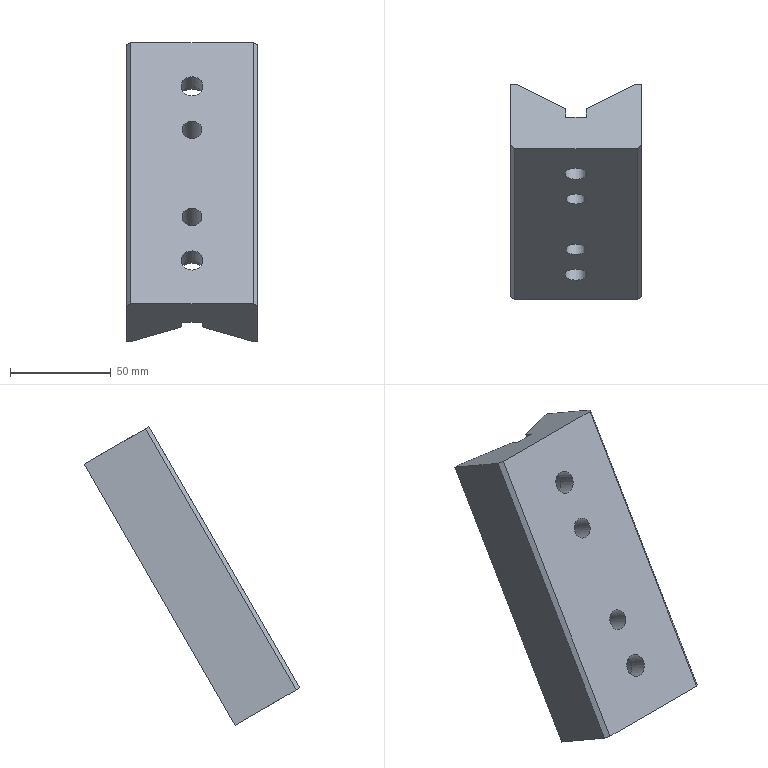Part | NX | features solid 2 | 1 solid | 30 faces | box 65 x 107.043 x 148.404 mm | volume 270452 mm3 | plane 24 | cylinder 6 | commonest cylinder face diameters 10 x2 11 x2 17.5 x2
STEP:
#1=CARTESIAN_POINT('',(-222.5,614.066,-72.467));
#2=VERTEX_POINT('',#1);
#3=CARTESIAN_POINT('',(-222.5,622.976,-57.036));
#4=VERTEX_POINT('',#3);
#5=CARTESIAN_POINT('',(-222.5,614.066,-72.467));
#6=DIRECTION('',(0.,0.5,0.866));
#7=VECTOR('',#6,1000.);
#8=LINE('',#5,#7);
#9=EDGE_CURVE('',#2,#4,#8,.T.);
#10=ORIENTED_EDGE('',*,*,#9,.F.);
#11=CARTESIAN_POINT('',(-222.5,618.298,-74.911));
#12=VERTEX_POINT('',#11);
#13=CARTESIAN_POINT('',(-222.5,614.066,-72.467));
#14=DIRECTION('',(0.,0.866,-0.5));
#15=VECTOR('',#14,1000.);
#16=LINE('',#13,#15);
#17=EDGE_CURVE('',#2,#12,#16,.T.);
#18=ORIENTED_EDGE('',*,*,#17,.T.);
#19=CARTESIAN_POINT('',(-222.5,627.208,-59.479));
#20=VERTEX_POINT('',#19);
#21=CARTESIAN_POINT('',(-222.5,618.298,-74.911));
#22=DIRECTION('',(0.,0.5,0.866));
#23=VECTOR('',#22,1000.);
#24=LINE('',#21,#23);
#25=EDGE_CURVE('',#12,#20,#24,.T.);
#26=ORIENTED_EDGE('',*,*,#25,.T.);
#27=CARTESIAN_POINT('',(-222.5,616.048,-53.036));
#28=DIRECTION('',(0.,0.866,-0.5));
#29=VECTOR('',#28,1000.);
#30=LINE('',#27,#29);
#31=EDGE_CURVE('',#4,#20,#30,.T.);
#32=ORIENTED_EDGE('',*,*,#31,.F.);
#33=EDGE_LOOP('',(#10,#18,#26,#32));
#34=FACE_BOUND('',#33,.T.);
#35=CARTESIAN_POINT('',(-222.5,614.066,-72.467));
#36=DIRECTION('',(-1.,0.,0.));
#37=DIRECTION('',(0.,-0.866,0.5));
#38=AXIS2_PLACEMENT_3D('',#35,#36,#37);
#39=PLANE('',#38);
#40=ADVANCED_FACE('',(#34),#39,.F.);
#41=CARTESIAN_POINT('',(-222.5,630.157,-44.598));
#42=VERTEX_POINT('',#41);
#43=CARTESIAN_POINT('',(-222.5,639.066,-29.166));
#44=VERTEX_POINT('',#43);
#45=CARTESIAN_POINT('',(-222.5,614.066,-72.467));
#46=DIRECTION('',(0.,0.5,0.866));
#47=VECTOR('',#46,1000.);
#48=LINE('',#45,#47);
#49=EDGE_CURVE('',#42,#44,#48,.T.);
#50=ORIENTED_EDGE('',*,*,#49,.T.);
#51=CARTESIAN_POINT('',(-212.5,639.066,-29.166));
#52=VERTEX_POINT('',#51);
#53=CARTESIAN_POINT('',(-217.5,639.066,-29.166));
#54=DIRECTION('',(0.,0.866,-0.5));
#55=DIRECTION('',(0.,-0.5,-0.866));
#56=AXIS2_PLACEMENT_3D('',#53,#54,#55);
#57=CIRCLE('',#56,5.);
#58=EDGE_CURVE('',#52,#44,#57,.T.);
#59=ORIENTED_EDGE('',*,*,#58,.F.);
#60=CARTESIAN_POINT('',(-212.5,630.157,-44.598));
#61=VERTEX_POINT('',#60);
#62=CARTESIAN_POINT('',(-212.5,614.066,-72.467));
#63=DIRECTION('',(0.,0.5,0.866));
#64=VECTOR('',#63,1000.);
#65=LINE('',#62,#64);
#66=EDGE_CURVE('',#61,#52,#65,.T.);
#67=ORIENTED_EDGE('',*,*,#66,.F.);
#68=CARTESIAN_POINT('',(-217.5,626.566,-50.817));
#69=DIRECTION('',(0.,0.866,-0.5));
#70=DIRECTION('',(0.,-0.5,-0.866));
#71=AXIS2_PLACEMENT_3D('',#68,#69,#70);
#72=CIRCLE('',#71,8.75);
#73=EDGE_CURVE('',#42,#61,#72,.T.);
#74=ORIENTED_EDGE('',*,*,#73,.F.);
#75=EDGE_LOOP('',(#50,#59,#67,#74));
#76=FACE_BOUND('',#75,.T.);
#77=CARTESIAN_POINT('',(-212.5,614.066,-72.467));
#78=DIRECTION('',(0.,-0.866,0.5));
#79=DIRECTION('',(0.,-0.5,-0.866));
#80=AXIS2_PLACEMENT_3D('',#77,#78,#79);
#81=PLANE('',#80);
#82=ADVANCED_FACE('',(#76),#81,.F.);
#83=ORIENTED_EDGE('',*,*,#66,.T.);
#84=CARTESIAN_POINT('',(-212.5,664.066,14.135));
#85=VERTEX_POINT('',#84);
#86=CARTESIAN_POINT('',(-212.5,614.066,-72.467));
#87=DIRECTION('',(0.,0.5,0.866));
#88=VECTOR('',#87,1000.);
#89=LINE('',#86,#88);
#90=EDGE_CURVE('',#52,#85,#89,.T.);
#91=ORIENTED_EDGE('',*,*,#90,.T.);
#92=CARTESIAN_POINT('',(-212.5,672.976,29.567));
#93=VERTEX_POINT('',#92);
#94=CARTESIAN_POINT('',(-212.5,614.066,-72.467));
#95=DIRECTION('',(0.,0.5,0.866));
#96=VECTOR('',#95,1000.);
#97=LINE('',#94,#96);
#98=EDGE_CURVE('',#85,#93,#97,.T.);
#99=ORIENTED_EDGE('',*,*,#98,.T.);
#100=CARTESIAN_POINT('',(-212.5,677.208,27.124));
#101=VERTEX_POINT('',#100);
#102=CARTESIAN_POINT('',(-212.5,666.048,33.567));
#103=DIRECTION('',(0.,0.866,-0.5));
#104=VECTOR('',#103,1000.);
#105=LINE('',#102,#104);
#106=EDGE_CURVE('',#101,#93,#105,.F.);
#107=ORIENTED_EDGE('',*,*,#106,.F.);
#108=CARTESIAN_POINT('',(-212.5,634.389,-47.042));
#109=VERTEX_POINT('',#108);
#110=CARTESIAN_POINT('',(-212.5,618.298,-74.911));
#111=DIRECTION('',(0.,0.5,0.866));
#112=VECTOR('',#111,1000.);
#113=LINE('',#110,#112);
#114=EDGE_CURVE('',#109,#101,#113,.T.);
#115=ORIENTED_EDGE('',*,*,#114,.F.);
#116=CARTESIAN_POINT('',(-212.5,623.228,-40.598));
#117=DIRECTION('',(0.,0.866,-0.5));
#118=VECTOR('',#117,1000.);
#119=LINE('',#116,#118);
#120=EDGE_CURVE('',#61,#109,#119,.T.);
#121=ORIENTED_EDGE('',*,*,#120,.F.);
#122=EDGE_LOOP('',(#83,#91,#99,#107,#115,#121));
#123=FACE_BOUND('',#122,.T.);
#124=CARTESIAN_POINT('',(-212.5,618.298,-74.911));
#125=DIRECTION('',(1.,0.,0.));
#126=DIRECTION('',(0.,0.866,-0.5));
#127=AXIS2_PLACEMENT_3D('',#124,#125,#126);
#128=PLANE('',#127);
#129=ADVANCED_FACE('',(#123),#128,.F.);
#130=CARTESIAN_POINT('',(-222.5,664.066,14.135));
#131=VERTEX_POINT('',#130);
#132=CARTESIAN_POINT('',(-222.5,614.066,-72.467));
#133=DIRECTION('',(0.,0.5,0.866));
#134=VECTOR('',#133,1000.);
#135=LINE('',#132,#134);
#136=EDGE_CURVE('',#44,#131,#135,.T.);
#137=ORIENTED_EDGE('',*,*,#136,.T.);
#138=CARTESIAN_POINT('',(-217.5,664.066,14.135));
#139=DIRECTION('',(0.,0.866,-0.5));
#140=DIRECTION('',(0.,-0.5,-0.866));
#141=AXIS2_PLACEMENT_3D('',#138,#139,#140);
#142=CIRCLE('',#141,5.);
#143=EDGE_CURVE('',#85,#131,#142,.T.);
#144=ORIENTED_EDGE('',*,*,#143,.F.);
#145=ORIENTED_EDGE('',*,*,#90,.F.);
#146=CARTESIAN_POINT('',(-217.5,639.066,-29.166));
#147=DIRECTION('',(0.,0.866,-0.5));
#148=DIRECTION('',(0.,-0.5,-0.866));
#149=AXIS2_PLACEMENT_3D('',#146,#147,#148);
#150=CIRCLE('',#149,5.);
#151=EDGE_CURVE('',#44,#52,#150,.T.);
#152=ORIENTED_EDGE('',*,*,#151,.F.);
#153=EDGE_LOOP('',(#137,#144,#145,#152));
#154=FACE_BOUND('',#153,.T.);
#155=CARTESIAN_POINT('',(-212.5,614.066,-72.467));
#156=DIRECTION('',(0.,-0.866,0.5));
#157=DIRECTION('',(0.,-0.5,-0.866));
#158=AXIS2_PLACEMENT_3D('',#155,#156,#157);
#159=PLANE('',#158);
#160=ADVANCED_FACE('',(#154),#159,.F.);
#161=CARTESIAN_POINT('',(-222.5,672.976,29.567));
#162=VERTEX_POINT('',#161);
#163=CARTESIAN_POINT('',(-222.5,614.066,-72.467));
#164=DIRECTION('',(0.,0.5,0.866));
#165=VECTOR('',#164,1000.);
#166=LINE('',#163,#165);
#167=EDGE_CURVE('',#131,#162,#166,.T.);
#168=ORIENTED_EDGE('',*,*,#167,.T.);
#169=CARTESIAN_POINT('',(-217.5,676.566,35.786));
#170=DIRECTION('',(0.,0.866,-0.5));
#171=DIRECTION('',(0.,-0.5,-0.866));
#172=AXIS2_PLACEMENT_3D('',#169,#170,#171);
#173=CIRCLE('',#172,8.75);
#174=EDGE_CURVE('',#93,#162,#173,.T.);
#175=ORIENTED_EDGE('',*,*,#174,.F.);
#176=ORIENTED_EDGE('',*,*,#98,.F.);
#177=CARTESIAN_POINT('',(-217.5,664.066,14.135));
#178=DIRECTION('',(0.,0.866,-0.5));
#179=DIRECTION('',(0.,-0.5,-0.866));
#180=AXIS2_PLACEMENT_3D('',#177,#178,#179);
#181=CIRCLE('',#180,5.);
#182=EDGE_CURVE('',#131,#85,#181,.T.);
#183=ORIENTED_EDGE('',*,*,#182,.F.);
#184=EDGE_LOOP('',(#168,#175,#176,#183));
#185=FACE_BOUND('',#184,.T.);
#186=CARTESIAN_POINT('',(-212.5,614.066,-72.467));
#187=DIRECTION('',(0.,-0.866,0.5));
#188=DIRECTION('',(0.,-0.5,-0.866));
#189=AXIS2_PLACEMENT_3D('',#186,#187,#188);
#190=PLANE('',#189);
#191=ADVANCED_FACE('',(#185),#190,.F.);
#192=CARTESIAN_POINT('',(-222.5,634.389,-47.042));
#193=VERTEX_POINT('',#192);
#194=CARTESIAN_POINT('',(-222.5,677.208,27.124));
#195=VERTEX_POINT('',#194);
#196=CARTESIAN_POINT('',(-222.5,618.298,-74.911));
#197=DIRECTION('',(0.,0.5,0.866));
#198=VECTOR('',#197,1000.);
#199=LINE('',#196,#198);
#200=EDGE_CURVE('',#193,#195,#199,.T.);
#201=ORIENTED_EDGE('',*,*,#200,.T.);
#202=CARTESIAN_POINT('',(-222.5,666.048,33.567));
#203=DIRECTION('',(0.,0.866,-0.5));
#204=VECTOR('',#203,1000.);
#205=LINE('',#202,#204);
#206=EDGE_CURVE('',#162,#195,#205,.T.);
#207=ORIENTED_EDGE('',*,*,#206,.F.);
#208=ORIENTED_EDGE('',*,*,#167,.F.);
#209=ORIENTED_EDGE('',*,*,#136,.F.);
#210=ORIENTED_EDGE('',*,*,#49,.F.);
#211=CARTESIAN_POINT('',(-222.5,623.228,-40.598));
#212=DIRECTION('',(0.,0.866,-0.5));
#213=VECTOR('',#212,1000.);
#214=LINE('',#211,#213);
#215=EDGE_CURVE('',#193,#42,#214,.F.);
#216=ORIENTED_EDGE('',*,*,#215,.F.);
#217=EDGE_LOOP('',(#201,#207,#208,#209,#210,#216));
#218=FACE_BOUND('',#217,.T.);
#219=CARTESIAN_POINT('',(-222.5,614.066,-72.467));
#220=DIRECTION('',(-1.,0.,0.));
#221=DIRECTION('',(0.,-0.866,0.5));
#222=AXIS2_PLACEMENT_3D('',#219,#220,#221);
#223=PLANE('',#222);
#224=ADVANCED_FACE('',(#218),#223,.F.);
#225=CARTESIAN_POINT('',(-222.5,680.157,42.004));
#226=VERTEX_POINT('',#225);
#227=CARTESIAN_POINT('',(-222.5,689.066,57.436));
#228=VERTEX_POINT('',#227);
#229=CARTESIAN_POINT('',(-222.5,614.066,-72.467));
#230=DIRECTION('',(0.,0.5,0.866));
#231=VECTOR('',#230,1000.);
#232=LINE('',#229,#231);
#233=EDGE_CURVE('',#226,#228,#232,.T.);
#234=ORIENTED_EDGE('',*,*,#233,.T.);
#235=CARTESIAN_POINT('',(-212.5,689.066,57.436));
#236=VERTEX_POINT('',#235);
#237=CARTESIAN_POINT('',(-212.5,689.066,57.436));
#238=DIRECTION('',(-1.,0.,0.));
#239=VECTOR('',#238,1000.);
#240=LINE('',#237,#239);
#241=EDGE_CURVE('',#236,#228,#240,.T.);
#242=ORIENTED_EDGE('',*,*,#241,.F.);
#243=CARTESIAN_POINT('',(-212.5,680.157,42.004));
#244=VERTEX_POINT('',#243);
#245=CARTESIAN_POINT('',(-212.5,614.066,-72.467));
#246=DIRECTION('',(0.,0.5,0.866));
#247=VECTOR('',#246,1000.);
#248=LINE('',#245,#247);
#249=EDGE_CURVE('',#244,#236,#248,.T.);
#250=ORIENTED_EDGE('',*,*,#249,.F.);
#251=CARTESIAN_POINT('',(-217.5,676.566,35.786));
#252=DIRECTION('',(0.,0.866,-0.5));
#253=DIRECTION('',(0.,-0.5,-0.866));
#254=AXIS2_PLACEMENT_3D('',#251,#252,#253);
#255=CIRCLE('',#254,8.75);
#256=EDGE_CURVE('',#226,#244,#255,.T.);
#257=ORIENTED_EDGE('',*,*,#256,.F.);
#258=EDGE_LOOP('',(#234,#242,#250,#257));
#259=FACE_BOUND('',#258,.T.);
#260=CARTESIAN_POINT('',(-212.5,614.066,-72.467));
#261=DIRECTION('',(0.,-0.866,0.5));
#262=DIRECTION('',(0.,-0.5,-0.866));
#263=AXIS2_PLACEMENT_3D('',#260,#261,#262);
#264=PLANE('',#263);
#265=ADVANCED_FACE('',(#259),#264,.F.);
#266=ORIENTED_EDGE('',*,*,#249,.T.);
#267=CARTESIAN_POINT('',(-212.5,693.298,54.993));
#268=VERTEX_POINT('',#267);
#269=CARTESIAN_POINT('',(-212.5,693.298,54.993));
#270=DIRECTION('',(0.,-0.866,0.5));
#271=VECTOR('',#270,1000.);
#272=LINE('',#269,#271);
#273=EDGE_CURVE('',#268,#236,#272,.T.);
#274=ORIENTED_EDGE('',*,*,#273,.F.);
#275=CARTESIAN_POINT('',(-212.5,684.389,39.561));
#276=VERTEX_POINT('',#275);
#277=CARTESIAN_POINT('',(-212.5,618.298,-74.911));
#278=DIRECTION('',(0.,0.5,0.866));
#279=VECTOR('',#278,1000.);
#280=LINE('',#277,#279);
#281=EDGE_CURVE('',#276,#268,#280,.T.);
#282=ORIENTED_EDGE('',*,*,#281,.F.);
#283=CARTESIAN_POINT('',(-212.5,673.228,46.004));
#284=DIRECTION('',(0.,0.866,-0.5));
#285=VECTOR('',#284,1000.);
#286=LINE('',#283,#285);
#287=EDGE_CURVE('',#244,#276,#286,.T.);
#288=ORIENTED_EDGE('',*,*,#287,.F.);
#289=EDGE_LOOP('',(#266,#274,#282,#288));
#290=FACE_BOUND('',#289,.T.);
#291=CARTESIAN_POINT('',(-212.5,618.298,-74.911));
#292=DIRECTION('',(1.,0.,0.));
#293=DIRECTION('',(0.,0.866,-0.5));
#294=AXIS2_PLACEMENT_3D('',#291,#292,#293);
#295=PLANE('',#294);
#296=ADVANCED_FACE('',(#290),#295,.F.);
#297=CARTESIAN_POINT('',(-217.5,613.728,-37.054));
#298=VERTEX_POINT('',#297);
#299=CARTESIAN_POINT('',(-217.5,610.978,-41.817));
#300=DIRECTION('',(0.,-0.866,0.5));
#301=DIRECTION('',(0.,0.5,0.866));
#302=AXIS2_PLACEMENT_3D('',#299,#300,#301);
#303=CIRCLE('',#302,5.5);
#304=EDGE_CURVE('',#298,#298,#303,.T.);
#305=ORIENTED_EDGE('',*,*,#304,.F.);
#306=EDGE_LOOP('',(#305));
#307=FACE_BOUND('',#306,.T.);
#308=CARTESIAN_POINT('',(-217.5,625.978,-15.836));
#309=VERTEX_POINT('',#308);
#310=CARTESIAN_POINT('',(-217.5,623.478,-20.166));
#311=DIRECTION('',(0.,-0.866,0.5));
#312=DIRECTION('',(0.,0.5,0.866));
#313=AXIS2_PLACEMENT_3D('',#310,#311,#312);
#314=CIRCLE('',#313,5.);
#315=EDGE_CURVE('',#309,#309,#314,.T.);
#316=ORIENTED_EDGE('',*,*,#315,.F.);
#317=EDGE_LOOP('',(#316));
#318=FACE_BOUND('',#317,.T.);
#319=CARTESIAN_POINT('',(-217.5,650.978,27.465));
#320=VERTEX_POINT('',#319);
#321=CARTESIAN_POINT('',(-217.5,648.478,23.135));
#322=DIRECTION('',(0.,-0.866,0.5));
#323=DIRECTION('',(0.,0.5,0.866));
#324=AXIS2_PLACEMENT_3D('',#321,#322,#323);
#325=CIRCLE('',#324,5.);
#326=EDGE_CURVE('',#320,#320,#325,.T.);
#327=ORIENTED_EDGE('',*,*,#326,.F.);
#328=EDGE_LOOP('',(#327));
#329=FACE_BOUND('',#328,.T.);
#330=CARTESIAN_POINT('',(-217.5,663.728,49.549));
#331=VERTEX_POINT('',#330);
#332=CARTESIAN_POINT('',(-217.5,660.978,44.786));
#333=DIRECTION('',(0.,-0.866,0.5));
#334=DIRECTION('',(0.,0.5,0.866));
#335=AXIS2_PLACEMENT_3D('',#332,#333,#334);
#336=CIRCLE('',#335,5.5);
#337=EDGE_CURVE('',#331,#331,#336,.T.);
#338=ORIENTED_EDGE('',*,*,#337,.F.);
#339=EDGE_LOOP('',(#338));
#340=FACE_BOUND('',#339,.T.);
#341=CARTESIAN_POINT('',(-187.,598.478,-63.467));
#342=VERTEX_POINT('',#341);
#343=CARTESIAN_POINT('',(-248.,598.478,-63.467));
#344=VERTEX_POINT('',#343);
#345=CARTESIAN_POINT('',(-185.,598.478,-63.467));
#346=DIRECTION('',(-1.,0.,0.));
#347=VECTOR('',#346,1000.);
#348=LINE('',#345,#347);
#349=EDGE_CURVE('',#342,#344,#348,.T.);
#350=ORIENTED_EDGE('',*,*,#349,.F.);
#351=CARTESIAN_POINT('',(-187.,673.478,66.436));
#352=VERTEX_POINT('',#351);
#353=CARTESIAN_POINT('',(-187.,598.478,-63.467));
#354=DIRECTION('',(0.,-0.5,-0.866));
#355=VECTOR('',#354,1000.);
#356=LINE('',#353,#355);
#357=EDGE_CURVE('',#352,#342,#356,.T.);
#358=ORIENTED_EDGE('',*,*,#357,.F.);
#359=CARTESIAN_POINT('',(-248.,673.478,66.436));
#360=VERTEX_POINT('',#359);
#361=CARTESIAN_POINT('',(-185.,673.478,66.436));
#362=DIRECTION('',(-1.,0.,0.));
#363=VECTOR('',#362,1000.);
#364=LINE('',#361,#363);
#365=EDGE_CURVE('',#352,#360,#364,.T.);
#366=ORIENTED_EDGE('',*,*,#365,.T.);
#367=CARTESIAN_POINT('',(-248.,598.478,-63.467));
#368=DIRECTION('',(0.,0.5,0.866));
#369=VECTOR('',#368,1000.);
#370=LINE('',#367,#369);
#371=EDGE_CURVE('',#344,#360,#370,.T.);
#372=ORIENTED_EDGE('',*,*,#371,.F.);
#373=EDGE_LOOP('',(#350,#358,#366,#372));
#374=FACE_BOUND('',#373,.T.);
#375=CARTESIAN_POINT('',(-185.,598.478,-63.467));
#376=DIRECTION('',(0.,-0.866,0.5));
#377=DIRECTION('',(1.,0.,0.));
#378=AXIS2_PLACEMENT_3D('',#375,#376,#377);
#379=PLANE('',#378);
#380=ADVANCED_FACE('',(#307,#318,#329,#340,#374),#379,.T.);
#381=CARTESIAN_POINT('',(-250.,675.21,65.436));
#382=VERTEX_POINT('',#381);
#383=CARTESIAN_POINT('',(-250.,705.521,47.936));
#384=VERTEX_POINT('',#383);
#385=CARTESIAN_POINT('',(-250.,673.478,66.436));
#386=DIRECTION('',(0.,0.866,-0.5));
#387=VECTOR('',#386,1000.);
#388=LINE('',#385,#387);
#389=EDGE_CURVE('',#382,#384,#388,.T.);
#390=ORIENTED_EDGE('',*,*,#389,.T.);
#391=CARTESIAN_POINT('',(-250.,630.521,-81.967));
#392=VERTEX_POINT('',#391);
#393=CARTESIAN_POINT('',(-250.,630.521,-81.967));
#394=DIRECTION('',(0.,0.5,0.866));
#395=VECTOR('',#394,1000.);
#396=LINE('',#393,#395);
#397=EDGE_CURVE('',#392,#384,#396,.T.);
#398=ORIENTED_EDGE('',*,*,#397,.F.);
#399=CARTESIAN_POINT('',(-250.,600.21,-64.467));
#400=VERTEX_POINT('',#399);
#401=CARTESIAN_POINT('',(-250.,598.478,-63.467));
#402=DIRECTION('',(0.,0.866,-0.5));
#403=VECTOR('',#402,1000.);
#404=LINE('',#401,#403);
#405=EDGE_CURVE('',#400,#392,#404,.T.);
#406=ORIENTED_EDGE('',*,*,#405,.F.);
#407=CARTESIAN_POINT('',(-250.,600.21,-64.467));
#408=DIRECTION('',(0.,-0.5,-0.866));
#409=VECTOR('',#408,1000.);
#410=LINE('',#407,#409);
#411=EDGE_CURVE('',#382,#400,#410,.T.);
#412=ORIENTED_EDGE('',*,*,#411,.F.);
#413=EDGE_LOOP('',(#390,#398,#406,#412));
#414=FACE_BOUND('',#413,.T.);
#415=CARTESIAN_POINT('',(-250.,598.478,-63.467));
#416=DIRECTION('',(-1.,0.,0.));
#417=DIRECTION('',(0.,-0.866,0.5));
#418=AXIS2_PLACEMENT_3D('',#415,#416,#417);
#419=PLANE('',#418);
#420=ADVANCED_FACE('',(#414),#419,.T.);
#421=CARTESIAN_POINT('',(-246.945,705.521,47.936));
#422=VERTEX_POINT('',#421);
#423=CARTESIAN_POINT('',(-250.,705.521,47.936));
#424=DIRECTION('',(1.,0.,0.));
#425=VECTOR('',#424,1000.);
#426=LINE('',#423,#425);
#427=EDGE_CURVE('',#384,#422,#426,.T.);
#428=ORIENTED_EDGE('',*,*,#427,.T.);
#429=CARTESIAN_POINT('',(-246.945,630.521,-81.967));
#430=VERTEX_POINT('',#429);
#431=CARTESIAN_POINT('',(-246.945,630.521,-81.967));
#432=DIRECTION('',(0.,0.5,0.866));
#433=VECTOR('',#432,1000.);
#434=LINE('',#431,#433);
#435=EDGE_CURVE('',#430,#422,#434,.T.);
#436=ORIENTED_EDGE('',*,*,#435,.F.);
#437=CARTESIAN_POINT('',(-250.,630.521,-81.967));
#438=DIRECTION('',(1.,0.,0.));
#439=VECTOR('',#438,1000.);
#440=LINE('',#437,#439);
#441=EDGE_CURVE('',#392,#430,#440,.T.);
#442=ORIENTED_EDGE('',*,*,#441,.F.);
#443=ORIENTED_EDGE('',*,*,#397,.T.);
#444=EDGE_LOOP('',(#428,#436,#442,#443));
#445=FACE_BOUND('',#444,.T.);
#446=CARTESIAN_POINT('',(-250.,630.521,-81.967));
#447=DIRECTION('',(0.,0.866,-0.5));
#448=DIRECTION('',(-1.,0.,0.));
#449=AXIS2_PLACEMENT_3D('',#446,#447,#448);
#450=PLANE('',#449);
#451=ADVANCED_FACE('',(#445),#450,.T.);
#452=ORIENTED_EDGE('',*,*,#25,.F.);
#453=CARTESIAN_POINT('',(-222.5,618.298,-74.911));
#454=DIRECTION('',(-0.866,0.433,-0.25));
#455=VECTOR('',#454,1000.);
#456=LINE('',#453,#455);
#457=EDGE_CURVE('',#12,#430,#456,.T.);
#458=ORIENTED_EDGE('',*,*,#457,.T.);
#459=ORIENTED_EDGE('',*,*,#435,.T.);
#460=CARTESIAN_POINT('',(-222.5,693.298,54.993));
#461=VERTEX_POINT('',#460);
#462=CARTESIAN_POINT('',(-222.5,693.298,54.993));
#463=DIRECTION('',(-0.866,0.433,-0.25));
#464=VECTOR('',#463,1000.);
#465=LINE('',#462,#464);
#466=EDGE_CURVE('',#461,#422,#465,.T.);
#467=ORIENTED_EDGE('',*,*,#466,.F.);
#468=CARTESIAN_POINT('',(-222.5,684.389,39.561));
#469=VERTEX_POINT('',#468);
#470=CARTESIAN_POINT('',(-222.5,618.298,-74.911));
#471=DIRECTION('',(0.,0.5,0.866));
#472=VECTOR('',#471,1000.);
#473=LINE('',#470,#472);
#474=EDGE_CURVE('',#469,#461,#473,.T.);
#475=ORIENTED_EDGE('',*,*,#474,.F.);
#476=CARTESIAN_POINT('',(-217.5,678.298,34.786));
#477=DIRECTION('',(0.5,0.75,-0.433));
#478=DIRECTION('',(-0.866,0.433,-0.25));
#479=AXIS2_PLACEMENT_3D('',#476,#477,#478);
#480=ELLIPSE('',#479,10.104,8.75);
#481=EDGE_CURVE('',#195,#469,#480,.T.);
#482=ORIENTED_EDGE('',*,*,#481,.F.);
#483=ORIENTED_EDGE('',*,*,#200,.F.);
#484=CARTESIAN_POINT('',(-217.5,628.298,-51.817));
#485=DIRECTION('',(0.5,0.75,-0.433));
#486=DIRECTION('',(-0.866,0.433,-0.25));
#487=AXIS2_PLACEMENT_3D('',#484,#485,#486);
#488=ELLIPSE('',#487,10.104,8.75);
#489=EDGE_CURVE('',#20,#193,#488,.T.);
#490=ORIENTED_EDGE('',*,*,#489,.F.);
#491=EDGE_LOOP('',(#452,#458,#459,#467,#475,#482,#483,#490));
#492=FACE_BOUND('',#491,.T.);
#493=CARTESIAN_POINT('',(-222.5,618.298,-74.911));
#494=DIRECTION('',(-0.5,-0.75,0.433));
#495=DIRECTION('',(0.866,-0.433,0.25));
#496=AXIS2_PLACEMENT_3D('',#493,#494,#495);
#497=PLANE('',#496);
#498=ADVANCED_FACE('',(#492),#497,.F.);
#499=ORIENTED_EDGE('',*,*,#474,.T.);
#500=CARTESIAN_POINT('',(-222.5,689.066,57.436));
#501=DIRECTION('',(0.,0.866,-0.5));
#502=VECTOR('',#501,1000.);
#503=LINE('',#500,#502);
#504=EDGE_CURVE('',#228,#461,#503,.T.);
#505=ORIENTED_EDGE('',*,*,#504,.F.);
#506=ORIENTED_EDGE('',*,*,#233,.F.);
#507=CARTESIAN_POINT('',(-222.5,673.228,46.004));
#508=DIRECTION('',(0.,0.866,-0.5));
#509=VECTOR('',#508,1000.);
#510=LINE('',#507,#509);
#511=EDGE_CURVE('',#469,#226,#510,.F.);
#512=ORIENTED_EDGE('',*,*,#511,.F.);
#513=EDGE_LOOP('',(#499,#505,#506,#512));
#514=FACE_BOUND('',#513,.T.);
#515=CARTESIAN_POINT('',(-222.5,614.066,-72.467));
#516=DIRECTION('',(-1.,0.,0.));
#517=DIRECTION('',(0.,-0.866,0.5));
#518=AXIS2_PLACEMENT_3D('',#515,#516,#517);
#519=PLANE('',#518);
#520=ADVANCED_FACE('',(#514),#519,.F.);
#521=CARTESIAN_POINT('',(-212.5,614.066,-72.467));
#522=VERTEX_POINT('',#521);
#523=CARTESIAN_POINT('',(-212.5,622.976,-57.036));
#524=VERTEX_POINT('',#523);
#525=CARTESIAN_POINT('',(-212.5,614.066,-72.467));
#526=DIRECTION('',(0.,0.5,0.866));
#527=VECTOR('',#526,1000.);
#528=LINE('',#525,#527);
#529=EDGE_CURVE('',#522,#524,#528,.T.);
#530=ORIENTED_EDGE('',*,*,#529,.F.);
#531=CARTESIAN_POINT('',(-212.5,614.066,-72.467));
#532=DIRECTION('',(-1.,0.,0.));
#533=VECTOR('',#532,1000.);
#534=LINE('',#531,#533);
#535=EDGE_CURVE('',#522,#2,#534,.T.);
#536=ORIENTED_EDGE('',*,*,#535,.T.);
#537=ORIENTED_EDGE('',*,*,#9,.T.);
#538=CARTESIAN_POINT('',(-217.5,626.566,-50.817));
#539=DIRECTION('',(0.,0.866,-0.5));
#540=DIRECTION('',(0.,-0.5,-0.866));
#541=AXIS2_PLACEMENT_3D('',#538,#539,#540);
#542=CIRCLE('',#541,8.75);
#543=EDGE_CURVE('',#524,#4,#542,.T.);
#544=ORIENTED_EDGE('',*,*,#543,.F.);
#545=EDGE_LOOP('',(#530,#536,#537,#544));
#546=FACE_BOUND('',#545,.T.);
#547=CARTESIAN_POINT('',(-212.5,614.066,-72.467));
#548=DIRECTION('',(0.,-0.866,0.5));
#549=DIRECTION('',(0.,-0.5,-0.866));
#550=AXIS2_PLACEMENT_3D('',#547,#548,#549);
#551=PLANE('',#550);
#552=ADVANCED_FACE('',(#546),#551,.F.);
#553=CARTESIAN_POINT('',(-212.5,618.298,-74.911));
#554=VERTEX_POINT('',#553);
#555=CARTESIAN_POINT('',(-212.5,627.208,-59.479));
#556=VERTEX_POINT('',#555);
#557=CARTESIAN_POINT('',(-212.5,618.298,-74.911));
#558=DIRECTION('',(0.,0.5,0.866));
#559=VECTOR('',#558,1000.);
#560=LINE('',#557,#559);
#561=EDGE_CURVE('',#554,#556,#560,.T.);
#562=ORIENTED_EDGE('',*,*,#561,.F.);
#563=CARTESIAN_POINT('',(-212.5,618.298,-74.911));
#564=DIRECTION('',(0.,-0.866,0.5));
#565=VECTOR('',#564,1000.);
#566=LINE('',#563,#565);
#567=EDGE_CURVE('',#554,#522,#566,.T.);
#568=ORIENTED_EDGE('',*,*,#567,.T.);
#569=ORIENTED_EDGE('',*,*,#529,.T.);
#570=CARTESIAN_POINT('',(-212.5,616.048,-53.036));
#571=DIRECTION('',(0.,0.866,-0.5));
#572=VECTOR('',#571,1000.);
#573=LINE('',#570,#572);
#574=EDGE_CURVE('',#556,#524,#573,.F.);
#575=ORIENTED_EDGE('',*,*,#574,.F.);
#576=EDGE_LOOP('',(#562,#568,#569,#575));
#577=FACE_BOUND('',#576,.T.);
#578=CARTESIAN_POINT('',(-212.5,618.298,-74.911));
#579=DIRECTION('',(1.,0.,0.));
#580=DIRECTION('',(0.,0.866,-0.5));
#581=AXIS2_PLACEMENT_3D('',#578,#579,#580);
#582=PLANE('',#581);
#583=ADVANCED_FACE('',(#577),#582,.F.);
#584=ORIENTED_EDGE('',*,*,#114,.T.);
#585=CARTESIAN_POINT('',(-217.5,678.298,34.786));
#586=DIRECTION('',(-0.5,0.75,-0.433));
#587=DIRECTION('',(0.866,0.433,-0.25));
#588=AXIS2_PLACEMENT_3D('',#585,#586,#587);
#589=ELLIPSE('',#588,10.104,8.75);
#590=EDGE_CURVE('',#276,#101,#589,.T.);
#591=ORIENTED_EDGE('',*,*,#590,.F.);
#592=ORIENTED_EDGE('',*,*,#281,.T.);
#593=CARTESIAN_POINT('',(-188.055,705.521,47.936));
#594=VERTEX_POINT('',#593);
#595=CARTESIAN_POINT('',(-188.055,705.521,47.936));
#596=DIRECTION('',(-0.866,-0.433,0.25));
#597=VECTOR('',#596,1000.);
#598=LINE('',#595,#597);
#599=EDGE_CURVE('',#594,#268,#598,.T.);
#600=ORIENTED_EDGE('',*,*,#599,.F.);
#601=CARTESIAN_POINT('',(-188.055,630.521,-81.967));
#602=VERTEX_POINT('',#601);
#603=CARTESIAN_POINT('',(-188.055,630.521,-81.967));
#604=DIRECTION('',(0.,0.5,0.866));
#605=VECTOR('',#604,1000.);
#606=LINE('',#603,#605);
#607=EDGE_CURVE('',#602,#594,#606,.T.);
#608=ORIENTED_EDGE('',*,*,#607,.F.);
#609=CARTESIAN_POINT('',(-188.055,630.521,-81.967));
#610=DIRECTION('',(-0.866,-0.433,0.25));
#611=VECTOR('',#610,1000.);
#612=LINE('',#609,#611);
#613=EDGE_CURVE('',#602,#554,#612,.T.);
#614=ORIENTED_EDGE('',*,*,#613,.T.);
#615=ORIENTED_EDGE('',*,*,#561,.T.);
#616=CARTESIAN_POINT('',(-217.5,628.298,-51.817));
#617=DIRECTION('',(-0.5,0.75,-0.433));
#618=DIRECTION('',(0.866,0.433,-0.25));
#619=AXIS2_PLACEMENT_3D('',#616,#617,#618);
#620=ELLIPSE('',#619,10.104,8.75);
#621=EDGE_CURVE('',#109,#556,#620,.T.);
#622=ORIENTED_EDGE('',*,*,#621,.F.);
#623=EDGE_LOOP('',(#584,#591,#592,#600,#608,#614,#615,#622));
#624=FACE_BOUND('',#623,.T.);
#625=CARTESIAN_POINT('',(-188.055,630.521,-81.967));
#626=DIRECTION('',(0.5,-0.75,0.433));
#627=DIRECTION('',(0.866,0.433,-0.25));
#628=AXIS2_PLACEMENT_3D('',#625,#626,#627);
#629=PLANE('',#628);
#630=ADVANCED_FACE('',(#624),#629,.F.);
#631=CARTESIAN_POINT('',(-185.,705.521,47.936));
#632=VERTEX_POINT('',#631);
#633=CARTESIAN_POINT('',(-188.055,705.521,47.936));
#634=DIRECTION('',(1.,0.,0.));
#635=VECTOR('',#634,1000.);
#636=LINE('',#633,#635);
#637=EDGE_CURVE('',#594,#632,#636,.T.);
#638=ORIENTED_EDGE('',*,*,#637,.T.);
#639=CARTESIAN_POINT('',(-185.,630.521,-81.967));
#640=VERTEX_POINT('',#639);
#641=CARTESIAN_POINT('',(-185.,630.521,-81.967));
#642=DIRECTION('',(0.,0.5,0.866));
#643=VECTOR('',#642,1000.);
#644=LINE('',#641,#643);
#645=EDGE_CURVE('',#640,#632,#644,.T.);
#646=ORIENTED_EDGE('',*,*,#645,.F.);
#647=CARTESIAN_POINT('',(-188.055,630.521,-81.967));
#648=DIRECTION('',(1.,0.,0.));
#649=VECTOR('',#648,1000.);
#650=LINE('',#647,#649);
#651=EDGE_CURVE('',#602,#640,#650,.T.);
#652=ORIENTED_EDGE('',*,*,#651,.F.);
#653=ORIENTED_EDGE('',*,*,#607,.T.);
#654=EDGE_LOOP('',(#638,#646,#652,#653));
#655=FACE_BOUND('',#654,.T.);
#656=CARTESIAN_POINT('',(-188.055,630.521,-81.967));
#657=DIRECTION('',(0.,0.866,-0.5));
#658=DIRECTION('',(-1.,0.,0.));
#659=AXIS2_PLACEMENT_3D('',#656,#657,#658);
#660=PLANE('',#659);
#661=ADVANCED_FACE('',(#655),#660,.T.);
#662=CARTESIAN_POINT('',(-185.,600.21,-64.467));
#663=VERTEX_POINT('',#662);
#664=CARTESIAN_POINT('',(-185.,630.521,-81.967));
#665=DIRECTION('',(0.,-0.866,0.5));
#666=VECTOR('',#665,1000.);
#667=LINE('',#664,#666);
#668=EDGE_CURVE('',#640,#663,#667,.T.);
#669=ORIENTED_EDGE('',*,*,#668,.F.);
#670=ORIENTED_EDGE('',*,*,#645,.T.);
#671=CARTESIAN_POINT('',(-185.,675.21,65.436));
#672=VERTEX_POINT('',#671);
#673=CARTESIAN_POINT('',(-185.,705.521,47.936));
#674=DIRECTION('',(0.,-0.866,0.5));
#675=VECTOR('',#674,1000.);
#676=LINE('',#673,#675);
#677=EDGE_CURVE('',#632,#672,#676,.T.);
#678=ORIENTED_EDGE('',*,*,#677,.T.);
#679=CARTESIAN_POINT('',(-185.,600.21,-64.467));
#680=DIRECTION('',(0.,0.5,0.866));
#681=VECTOR('',#680,1000.);
#682=LINE('',#679,#681);
#683=EDGE_CURVE('',#663,#672,#682,.T.);
#684=ORIENTED_EDGE('',*,*,#683,.F.);
#685=EDGE_LOOP('',(#669,#670,#678,#684));
#686=FACE_BOUND('',#685,.T.);
#687=CARTESIAN_POINT('',(-185.,630.521,-81.967));
#688=DIRECTION('',(1.,0.,0.));
#689=DIRECTION('',(0.,0.866,-0.5));
#690=AXIS2_PLACEMENT_3D('',#687,#688,#689);
#691=PLANE('',#690);
#692=ADVANCED_FACE('',(#686),#691,.T.);
#693=ORIENTED_EDGE('',*,*,#405,.T.);
#694=ORIENTED_EDGE('',*,*,#441,.T.);
#695=ORIENTED_EDGE('',*,*,#457,.F.);
#696=ORIENTED_EDGE('',*,*,#17,.F.);
#697=ORIENTED_EDGE('',*,*,#535,.F.);
#698=ORIENTED_EDGE('',*,*,#567,.F.);
#699=ORIENTED_EDGE('',*,*,#613,.F.);
#700=ORIENTED_EDGE('',*,*,#651,.T.);
#701=ORIENTED_EDGE('',*,*,#668,.T.);
#702=CARTESIAN_POINT('',(-185.,600.21,-64.467));
#703=DIRECTION('',(-0.7071,-0.6124,0.3536));
#704=VECTOR('',#703,1000.);
#705=LINE('',#702,#704);
#706=EDGE_CURVE('',#342,#663,#705,.F.);
#707=ORIENTED_EDGE('',*,*,#706,.F.);
#708=ORIENTED_EDGE('',*,*,#349,.T.);
#709=CARTESIAN_POINT('',(-248.,598.478,-63.467));
#710=DIRECTION('',(-0.7071,0.6124,-0.3536));
#711=VECTOR('',#710,1000.);
#712=LINE('',#709,#711);
#713=EDGE_CURVE('',#400,#344,#712,.F.);
#714=ORIENTED_EDGE('',*,*,#713,.F.);
#715=EDGE_LOOP('',(#693,#694,#695,#696,#697,#698,#699,#700,#701,#707,#708,#714));
#716=FACE_BOUND('',#715,.T.);
#717=CARTESIAN_POINT('',(-222.5,598.478,-63.467));
#718=DIRECTION('',(0.,0.5,0.866));
#719=DIRECTION('',(0.,-0.866,0.5));
#720=AXIS2_PLACEMENT_3D('',#717,#718,#719);
#721=PLANE('',#720);
#722=ADVANCED_FACE('',(#716),#721,.F.);
#723=ORIENTED_EDGE('',*,*,#365,.F.);
#724=CARTESIAN_POINT('',(-204.75,658.106,75.311));
#725=DIRECTION('',(0.7071,0.6124,-0.3536));
#726=VECTOR('',#725,1000.);
#727=LINE('',#724,#726);
#728=EDGE_CURVE('',#672,#352,#727,.F.);
#729=ORIENTED_EDGE('',*,*,#728,.F.);
#730=ORIENTED_EDGE('',*,*,#677,.F.);
#731=ORIENTED_EDGE('',*,*,#637,.F.);
#732=ORIENTED_EDGE('',*,*,#599,.T.);
#733=ORIENTED_EDGE('',*,*,#273,.T.);
#734=ORIENTED_EDGE('',*,*,#241,.T.);
#735=ORIENTED_EDGE('',*,*,#504,.T.);
#736=ORIENTED_EDGE('',*,*,#466,.T.);
#737=ORIENTED_EDGE('',*,*,#427,.F.);
#738=ORIENTED_EDGE('',*,*,#389,.F.);
#739=CARTESIAN_POINT('',(-235.25,662.436,72.811));
#740=DIRECTION('',(0.7071,-0.6124,0.3536));
#741=VECTOR('',#740,1000.);
#742=LINE('',#739,#741);
#743=EDGE_CURVE('',#360,#382,#742,.F.);
#744=ORIENTED_EDGE('',*,*,#743,.F.);
#745=EDGE_LOOP('',(#723,#729,#730,#731,#732,#733,#734,#735,#736,#737,#738,#744));
#746=FACE_BOUND('',#745,.T.);
#747=CARTESIAN_POINT('',(-222.5,673.478,66.436));
#748=DIRECTION('',(0.,0.5,0.866));
#749=DIRECTION('',(0.,-0.866,0.5));
#750=AXIS2_PLACEMENT_3D('',#747,#748,#749);
#751=PLANE('',#750);
#752=ADVANCED_FACE('',(#746),#751,.T.);
#753=CARTESIAN_POINT('',(-217.5,666.888,35.023));
#754=VERTEX_POINT('',#753);
#755=CARTESIAN_POINT('',(-217.5,669.638,39.786));
#756=DIRECTION('',(0.,0.866,-0.5));
#757=DIRECTION('',(0.,-0.5,-0.866));
#758=AXIS2_PLACEMENT_3D('',#755,#756,#757);
#759=CIRCLE('',#758,5.5);
#760=EDGE_CURVE('',#754,#754,#759,.F.);
#761=ORIENTED_EDGE('',*,*,#760,.F.);
#762=EDGE_LOOP('',(#761));
#763=FACE_BOUND('',#762,.T.);
#764=ORIENTED_EDGE('',*,*,#337,.T.);
#765=EDGE_LOOP('',(#764));
#766=FACE_BOUND('',#765,.T.);
#767=CARTESIAN_POINT('',(-217.5,660.978,44.786));
#768=DIRECTION('',(0.,0.866,-0.5));
#769=DIRECTION('',(0.,0.5,0.866));
#770=AXIS2_PLACEMENT_3D('',#767,#768,#769);
#771=CYLINDRICAL_SURFACE('',#770,5.5);
#772=ADVANCED_FACE('',(#763,#766),#771,.F.);
#773=CARTESIAN_POINT('',(-217.5,674.013,47.363));
#774=VERTEX_POINT('',#773);
#775=CARTESIAN_POINT('',(-217.5,669.638,39.786));
#776=DIRECTION('',(0.,-0.866,0.5));
#777=DIRECTION('',(0.,0.5,0.866));
#778=AXIS2_PLACEMENT_3D('',#775,#776,#777);
#779=CIRCLE('',#778,8.75);
#780=EDGE_CURVE('',#774,#774,#779,.T.);
#781=ORIENTED_EDGE('',*,*,#780,.T.);
#782=EDGE_LOOP('',(#781));
#783=FACE_BOUND('',#782,.T.);
#784=ORIENTED_EDGE('',*,*,#206,.T.);
#785=ORIENTED_EDGE('',*,*,#481,.T.);
#786=ORIENTED_EDGE('',*,*,#511,.T.);
#787=ORIENTED_EDGE('',*,*,#256,.T.);
#788=ORIENTED_EDGE('',*,*,#287,.T.);
#789=ORIENTED_EDGE('',*,*,#590,.T.);
#790=ORIENTED_EDGE('',*,*,#106,.T.);
#791=ORIENTED_EDGE('',*,*,#174,.T.);
#792=EDGE_LOOP('',(#784,#785,#786,#787,#788,#789,#790,#791));
#793=FACE_BOUND('',#792,.T.);
#794=CARTESIAN_POINT('',(-217.5,669.638,39.786));
#795=DIRECTION('',(0.,0.866,-0.5));
#796=DIRECTION('',(0.,0.5,0.866));
#797=AXIS2_PLACEMENT_3D('',#794,#795,#796);
#798=CYLINDRICAL_SURFACE('',#797,8.75);
#799=ADVANCED_FACE('',(#783,#793),#798,.F.);
#800=ORIENTED_EDGE('',*,*,#780,.F.);
#801=EDGE_LOOP('',(#800));
#802=FACE_BOUND('',#801,.T.);
#803=ORIENTED_EDGE('',*,*,#760,.T.);
#804=EDGE_LOOP('',(#803));
#805=FACE_BOUND('',#804,.T.);
#806=CARTESIAN_POINT('',(-217.5,669.638,39.786));
#807=DIRECTION('',(0.,-0.866,0.5));
#808=DIRECTION('',(0.,-0.5,-0.866));
#809=AXIS2_PLACEMENT_3D('',#806,#807,#808);
#810=PLANE('',#809);
#811=ADVANCED_FACE('',(#802,#805),#810,.F.);
#812=ORIENTED_EDGE('',*,*,#326,.T.);
#813=EDGE_LOOP('',(#812));
#814=FACE_BOUND('',#813,.T.);
#815=ORIENTED_EDGE('',*,*,#143,.T.);
#816=ORIENTED_EDGE('',*,*,#182,.T.);
#817=EDGE_LOOP('',(#815,#816));
#818=FACE_BOUND('',#817,.T.);
#819=CARTESIAN_POINT('',(-217.5,648.478,23.135));
#820=DIRECTION('',(0.,0.866,-0.5));
#821=DIRECTION('',(0.,0.5,0.866));
#822=AXIS2_PLACEMENT_3D('',#819,#820,#821);
#823=CYLINDRICAL_SURFACE('',#822,5.);
#824=ADVANCED_FACE('',(#814,#818),#823,.F.);
#825=ORIENTED_EDGE('',*,*,#315,.T.);
#826=EDGE_LOOP('',(#825));
#827=FACE_BOUND('',#826,.T.);
#828=ORIENTED_EDGE('',*,*,#58,.T.);
#829=ORIENTED_EDGE('',*,*,#151,.T.);
#830=EDGE_LOOP('',(#828,#829));
#831=FACE_BOUND('',#830,.T.);
#832=CARTESIAN_POINT('',(-217.5,623.478,-20.166));
#833=DIRECTION('',(0.,0.866,-0.5));
#834=DIRECTION('',(0.,0.5,0.866));
#835=AXIS2_PLACEMENT_3D('',#832,#833,#834);
#836=CYLINDRICAL_SURFACE('',#835,5.);
#837=ADVANCED_FACE('',(#827,#831),#836,.F.);
#838=CARTESIAN_POINT('',(-217.5,616.888,-51.58));
#839=VERTEX_POINT('',#838);
#840=CARTESIAN_POINT('',(-217.5,619.638,-46.817));
#841=DIRECTION('',(0.,0.866,-0.5));
#842=DIRECTION('',(0.,-0.5,-0.866));
#843=AXIS2_PLACEMENT_3D('',#840,#841,#842);
#844=CIRCLE('',#843,5.5);
#845=EDGE_CURVE('',#839,#839,#844,.F.);
#846=ORIENTED_EDGE('',*,*,#845,.F.);
#847=EDGE_LOOP('',(#846));
#848=FACE_BOUND('',#847,.T.);
#849=ORIENTED_EDGE('',*,*,#304,.T.);
#850=EDGE_LOOP('',(#849));
#851=FACE_BOUND('',#850,.T.);
#852=CARTESIAN_POINT('',(-217.5,610.978,-41.817));
#853=DIRECTION('',(0.,0.866,-0.5));
#854=DIRECTION('',(0.,0.5,0.866));
#855=AXIS2_PLACEMENT_3D('',#852,#853,#854);
#856=CYLINDRICAL_SURFACE('',#855,5.5);
#857=ADVANCED_FACE('',(#848,#851),#856,.F.);
#858=CARTESIAN_POINT('',(-217.5,624.013,-39.239));
#859=VERTEX_POINT('',#858);
#860=CARTESIAN_POINT('',(-217.5,619.638,-46.817));
#861=DIRECTION('',(0.,-0.866,0.5));
#862=DIRECTION('',(0.,0.5,0.866));
#863=AXIS2_PLACEMENT_3D('',#860,#861,#862);
#864=CIRCLE('',#863,8.75);
#865=EDGE_CURVE('',#859,#859,#864,.T.);
#866=ORIENTED_EDGE('',*,*,#865,.T.);
#867=EDGE_LOOP('',(#866));
#868=FACE_BOUND('',#867,.T.);
#869=ORIENTED_EDGE('',*,*,#31,.T.);
#870=ORIENTED_EDGE('',*,*,#489,.T.);
#871=ORIENTED_EDGE('',*,*,#215,.T.);
#872=ORIENTED_EDGE('',*,*,#73,.T.);
#873=ORIENTED_EDGE('',*,*,#120,.T.);
#874=ORIENTED_EDGE('',*,*,#621,.T.);
#875=ORIENTED_EDGE('',*,*,#574,.T.);
#876=ORIENTED_EDGE('',*,*,#543,.T.);
#877=EDGE_LOOP('',(#869,#870,#871,#872,#873,#874,#875,#876));
#878=FACE_BOUND('',#877,.T.);
#879=CARTESIAN_POINT('',(-217.5,619.638,-46.817));
#880=DIRECTION('',(0.,0.866,-0.5));
#881=DIRECTION('',(0.,0.5,0.866));
#882=AXIS2_PLACEMENT_3D('',#879,#880,#881);
#883=CYLINDRICAL_SURFACE('',#882,8.75);
#884=ADVANCED_FACE('',(#868,#878),#883,.F.);
#885=ORIENTED_EDGE('',*,*,#865,.F.);
#886=EDGE_LOOP('',(#885));
#887=FACE_BOUND('',#886,.T.);
#888=ORIENTED_EDGE('',*,*,#845,.T.);
#889=EDGE_LOOP('',(#888));
#890=FACE_BOUND('',#889,.T.);
#891=CARTESIAN_POINT('',(-217.5,619.638,-46.817));
#892=DIRECTION('',(0.,-0.866,0.5));
#893=DIRECTION('',(0.,-0.5,-0.866));
#894=AXIS2_PLACEMENT_3D('',#891,#892,#893);
#895=PLANE('',#894);
#896=ADVANCED_FACE('',(#887,#890),#895,.F.);
#897=ORIENTED_EDGE('',*,*,#713,.T.);
#898=ORIENTED_EDGE('',*,*,#371,.T.);
#899=ORIENTED_EDGE('',*,*,#743,.T.);
#900=ORIENTED_EDGE('',*,*,#411,.T.);
#901=EDGE_LOOP('',(#897,#898,#899,#900));
#902=FACE_BOUND('',#901,.T.);
#903=CARTESIAN_POINT('',(-248.,598.478,-63.467));
#904=DIRECTION('',(0.7071,0.6124,-0.3536));
#905=DIRECTION('',(-0.7071,0.6124,-0.3536));
#906=AXIS2_PLACEMENT_3D('',#903,#904,#905);
#907=PLANE('',#906);
#908=ADVANCED_FACE('',(#902),#907,.F.);
#909=ORIENTED_EDGE('',*,*,#706,.T.);
#910=ORIENTED_EDGE('',*,*,#683,.T.);
#911=ORIENTED_EDGE('',*,*,#728,.T.);
#912=ORIENTED_EDGE('',*,*,#357,.T.);
#913=EDGE_LOOP('',(#909,#910,#911,#912));
#914=FACE_BOUND('',#913,.T.);
#915=CARTESIAN_POINT('',(-185.,600.21,-64.467));
#916=DIRECTION('',(-0.7071,0.6124,-0.3536));
#917=DIRECTION('',(-0.7071,-0.6124,0.3536));
#918=AXIS2_PLACEMENT_3D('',#915,#916,#917);
#919=PLANE('',#918);
#920=ADVANCED_FACE('',(#914),#919,.F.);
#921=CLOSED_SHELL('',(#40,#82,#129,#160,#191,#224,#265,#296,#380,#420,#451,#498,#520,#552,#583,#630,#661,#692,#722,#752,#772,#799,#811,#824,#837,#857,#884,#896,#908,#920));
#922=MANIFOLD_SOLID_BREP('',#921);
#923=(LENGTH_UNIT()NAMED_UNIT(*)SI_UNIT(.MILLI.,.METRE.));
#924=UNCERTAINTY_MEASURE_WITH_UNIT(LENGTH_MEASURE(0.00001),#923,'','');
#925=(NAMED_UNIT(*)PLANE_ANGLE_UNIT()SI_UNIT($,.RADIAN.));
#926=(NAMED_UNIT(*)SI_UNIT($,.STERADIAN.)SOLID_ANGLE_UNIT());
#927=(GEOMETRIC_REPRESENTATION_CONTEXT(3)GLOBAL_UNCERTAINTY_ASSIGNED_CONTEXT((#924))GLOBAL_UNIT_ASSIGNED_CONTEXT((#923,#925,#926))REPRESENTATION_CONTEXT('',''));
#928=ADVANCED_BREP_SHAPE_REPRESENTATION('',(#922),#927);